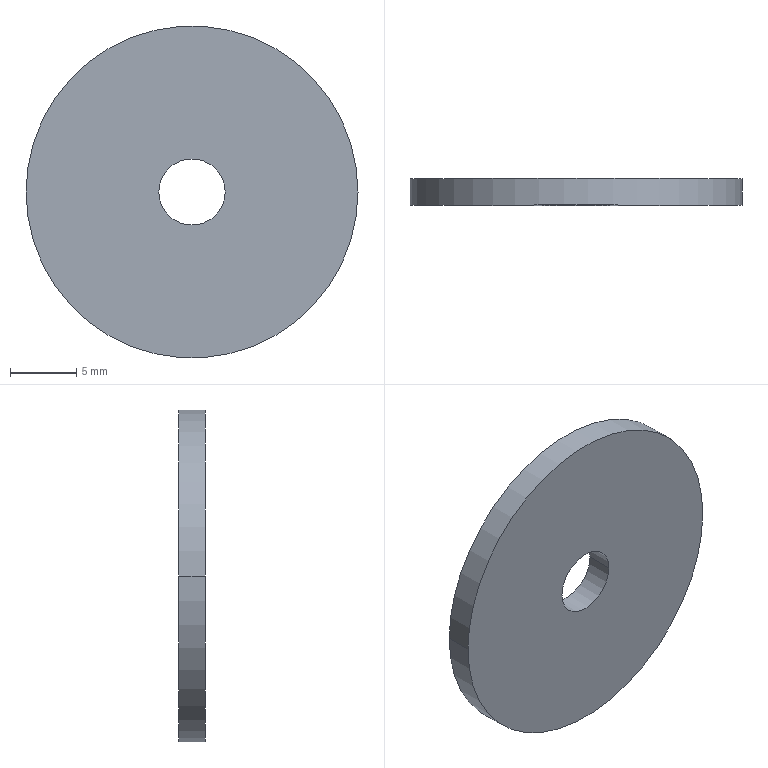Part | STEP file | BAR_INSUL_25 | 1 solid | 6 faces | box 25 x 2 x 25 mm | volume 942.478 mm3 | cylinder 4 | plane 2 | commonest cylinder face diameters 5 x2 25 x2
STEP:
#1=CARTESIAN_POINT('',(0.,0.,0.));
#2=DIRECTION('',(0.,0.,1.));
#3=DIRECTION('',(1.,0.,0.));
#4=AXIS2_PLACEMENT_3D('',#1,#2,#3);
#5=CARTESIAN_POINT('',(-12.5,0.,0.));
#6=VERTEX_POINT('',#5);
#7=CARTESIAN_POINT('',(12.5,0.,0.));
#8=VERTEX_POINT('',#7);
#9=CARTESIAN_POINT('',(0.,0.,0.));
#10=DIRECTION('',(0.,1.,0.));
#11=DIRECTION('',(-1.,0.,0.));
#12=AXIS2_PLACEMENT_3D('',#9,#10,#11);
#13=CIRCLE('',#12,12.5);
#14=CARTESIAN_POINT('',(0.,0.,0.));
#15=DIRECTION('',(0.,1.,0.));
#16=DIRECTION('',(-1.,0.,0.));
#17=AXIS2_PLACEMENT_3D('',#14,#15,#16);
#18=PLANE('',#17);
#19=CARTESIAN_POINT('',(0.,0.));
#20=DIRECTION('',(1.,0.));
#21=AXIS2_PLACEMENT_2D('',#19,#20);
#22=CIRCLE('',#21,12.5);
#23=(GEOMETRIC_REPRESENTATION_CONTEXT(2)PARAMETRIC_REPRESENTATION_CONTEXT()REPRESENTATION_CONTEXT('',''));
#24=DEFINITIONAL_REPRESENTATION('',(#22),#23);
#25=PCURVE('',#18,#24);
#26=CARTESIAN_POINT('',(0.,0.,0.));
#27=DIRECTION('',(0.,1.,0.));
#28=DIRECTION('',(-1.,0.,0.));
#29=AXIS2_PLACEMENT_3D('',#26,#27,#28);
#30=CYLINDRICAL_SURFACE('',#29,12.5);
#31=CARTESIAN_POINT('',(0.,0.));
#32=DIRECTION('',(1.,0.));
#33=VECTOR('',#32,1.);
#34=LINE('',#31,#33);
#35=(GEOMETRIC_REPRESENTATION_CONTEXT(2)PARAMETRIC_REPRESENTATION_CONTEXT()REPRESENTATION_CONTEXT('',''));
#36=DEFINITIONAL_REPRESENTATION('',(#34),#35);
#37=PCURVE('',#30,#36);
#38=SURFACE_CURVE('',#13,(#25,#37),.PCURVE_S1.);
#39=EDGE_CURVE('',#6,#8,#38,.T.);
#40=ORIENTED_EDGE('',*,*,#39,.T.);
#41=CARTESIAN_POINT('',(0.,0.,0.));
#42=DIRECTION('',(0.,1.,0.));
#43=DIRECTION('',(1.,0.,0.));
#44=AXIS2_PLACEMENT_3D('',#41,#42,#43);
#45=CIRCLE('',#44,12.5);
#46=CARTESIAN_POINT('',(0.,0.));
#47=DIRECTION('',(-1.,0.));
#48=AXIS2_PLACEMENT_2D('',#46,#47);
#49=CIRCLE('',#48,12.5);
#50=(GEOMETRIC_REPRESENTATION_CONTEXT(2)PARAMETRIC_REPRESENTATION_CONTEXT()REPRESENTATION_CONTEXT('',''));
#51=DEFINITIONAL_REPRESENTATION('',(#49),#50);
#52=PCURVE('',#18,#51);
#53=CARTESIAN_POINT('',(0.,0.,0.));
#54=DIRECTION('',(0.,1.,0.));
#55=DIRECTION('',(-1.,0.,0.));
#56=AXIS2_PLACEMENT_3D('',#53,#54,#55);
#57=CYLINDRICAL_SURFACE('',#56,12.5);
#58=CARTESIAN_POINT('',(3.142,0.));
#59=DIRECTION('',(1.,0.));
#60=VECTOR('',#59,1.);
#61=LINE('',#58,#60);
#62=(GEOMETRIC_REPRESENTATION_CONTEXT(2)PARAMETRIC_REPRESENTATION_CONTEXT()REPRESENTATION_CONTEXT('',''));
#63=DEFINITIONAL_REPRESENTATION('',(#61),#62);
#64=PCURVE('',#57,#63);
#65=SURFACE_CURVE('',#45,(#52,#64),.PCURVE_S1.);
#66=EDGE_CURVE('',#8,#6,#65,.T.);
#67=ORIENTED_EDGE('',*,*,#66,.T.);
#68=EDGE_LOOP('',(#40,#67));
#69=FACE_BOUND('',#68,.F.);
#70=CARTESIAN_POINT('',(-2.5,0.,0.));
#71=VERTEX_POINT('',#70);
#72=CARTESIAN_POINT('',(2.5,0.,0.));
#73=VERTEX_POINT('',#72);
#74=CARTESIAN_POINT('',(0.,0.,0.));
#75=DIRECTION('',(0.,-1.,0.));
#76=DIRECTION('',(-1.,0.,0.));
#77=AXIS2_PLACEMENT_3D('',#74,#75,#76);
#78=CIRCLE('',#77,2.5);
#79=CARTESIAN_POINT('',(2.5,0.));
#80=CARTESIAN_POINT('',(2.5,-4.33));
#81=CARTESIAN_POINT('',(-1.25,-2.165));
#82=CARTESIAN_POINT('',(-5.,0.));
#83=CARTESIAN_POINT('',(-1.25,2.165));
#84=CARTESIAN_POINT('',(2.5,4.33));
#85=CARTESIAN_POINT('',(2.5,0.));
#86=(BOUNDED_CURVE()B_SPLINE_CURVE(2,(#79,#80,#81,#82,#83,#84,#85),.UNSPECIFIED.,.T.,.F.)B_SPLINE_CURVE_WITH_KNOTS((1,2,2,2,2,1),(-2.094,0.,2.094,4.189,6.283,8.378),.UNSPECIFIED.)CURVE()GEOMETRIC_REPRESENTATION_ITEM()RATIONAL_B_SPLINE_CURVE((1.,0.5,1.,0.5,1.,0.5,1.))REPRESENTATION_ITEM(''));
#87=(GEOMETRIC_REPRESENTATION_CONTEXT(2)PARAMETRIC_REPRESENTATION_CONTEXT()REPRESENTATION_CONTEXT('',''));
#88=DEFINITIONAL_REPRESENTATION('',(#86),#87);
#89=PCURVE('',#18,#88);
#90=CARTESIAN_POINT('',(0.,0.,0.));
#91=DIRECTION('',(0.,1.,0.));
#92=DIRECTION('',(-1.,0.,0.));
#93=AXIS2_PLACEMENT_3D('',#90,#91,#92);
#94=CYLINDRICAL_SURFACE('',#93,2.5);
#95=CARTESIAN_POINT('',(6.283,0.));
#96=DIRECTION('',(-1.,0.));
#97=VECTOR('',#96,1.);
#98=LINE('',#95,#97);
#99=(GEOMETRIC_REPRESENTATION_CONTEXT(2)PARAMETRIC_REPRESENTATION_CONTEXT()REPRESENTATION_CONTEXT('',''));
#100=DEFINITIONAL_REPRESENTATION('',(#98),#99);
#101=PCURVE('',#94,#100);
#102=SURFACE_CURVE('',#78,(#89,#101),.PCURVE_S1.);
#103=EDGE_CURVE('',#71,#73,#102,.T.);
#104=ORIENTED_EDGE('',*,*,#103,.T.);
#105=CARTESIAN_POINT('',(0.,0.,0.));
#106=DIRECTION('',(0.,-1.,0.));
#107=DIRECTION('',(1.,0.,0.));
#108=AXIS2_PLACEMENT_3D('',#105,#106,#107);
#109=CIRCLE('',#108,2.5);
#110=CARTESIAN_POINT('',(-2.5,0.));
#111=CARTESIAN_POINT('',(-2.5,4.33));
#112=CARTESIAN_POINT('',(1.25,2.165));
#113=CARTESIAN_POINT('',(5.,0.));
#114=CARTESIAN_POINT('',(1.25,-2.165));
#115=CARTESIAN_POINT('',(-2.5,-4.33));
#116=CARTESIAN_POINT('',(-2.5,0.));
#117=(BOUNDED_CURVE()B_SPLINE_CURVE(2,(#110,#111,#112,#113,#114,#115,#116),.UNSPECIFIED.,.T.,.F.)B_SPLINE_CURVE_WITH_KNOTS((1,2,2,2,2,1),(-2.094,0.,2.094,4.189,6.283,8.378),.UNSPECIFIED.)CURVE()GEOMETRIC_REPRESENTATION_ITEM()RATIONAL_B_SPLINE_CURVE((1.,0.5,1.,0.5,1.,0.5,1.))REPRESENTATION_ITEM(''));
#118=(GEOMETRIC_REPRESENTATION_CONTEXT(2)PARAMETRIC_REPRESENTATION_CONTEXT()REPRESENTATION_CONTEXT('',''));
#119=DEFINITIONAL_REPRESENTATION('',(#117),#118);
#120=PCURVE('',#18,#119);
#121=CARTESIAN_POINT('',(0.,0.,0.));
#122=DIRECTION('',(0.,1.,0.));
#123=DIRECTION('',(-1.,0.,0.));
#124=AXIS2_PLACEMENT_3D('',#121,#122,#123);
#125=CYLINDRICAL_SURFACE('',#124,2.5);
#126=CARTESIAN_POINT('',(3.142,0.));
#127=DIRECTION('',(-1.,0.));
#128=VECTOR('',#127,1.);
#129=LINE('',#126,#128);
#130=(GEOMETRIC_REPRESENTATION_CONTEXT(2)PARAMETRIC_REPRESENTATION_CONTEXT()REPRESENTATION_CONTEXT('',''));
#131=DEFINITIONAL_REPRESENTATION('',(#129),#130);
#132=PCURVE('',#125,#131);
#133=SURFACE_CURVE('',#109,(#120,#132),.PCURVE_S1.);
#134=EDGE_CURVE('',#73,#71,#133,.T.);
#135=ORIENTED_EDGE('',*,*,#134,.T.);
#136=EDGE_LOOP('',(#104,#135));
#137=FACE_BOUND('',#136,.F.);
#138=ADVANCED_FACE('',(#69,#137),#18,.F.);
#139=CARTESIAN_POINT('',(12.5,2.,0.));
#140=VERTEX_POINT('',#139);
#141=CARTESIAN_POINT('',(12.5,0.,0.));
#142=DIRECTION('',(0.,1.,0.));
#143=VECTOR('',#142,1.);
#144=LINE('',#141,#143);
#145=CARTESIAN_POINT('',(3.142,0.));
#146=DIRECTION('',(0.,1.));
#147=VECTOR('',#146,1.);
#148=LINE('',#145,#147);
#149=(GEOMETRIC_REPRESENTATION_CONTEXT(2)PARAMETRIC_REPRESENTATION_CONTEXT()REPRESENTATION_CONTEXT('',''));
#150=DEFINITIONAL_REPRESENTATION('',(#148),#149);
#151=PCURVE('',#30,#150);
#152=CARTESIAN_POINT('',(3.142,0.));
#153=DIRECTION('',(0.,1.));
#154=VECTOR('',#153,1.);
#155=LINE('',#152,#154);
#156=(GEOMETRIC_REPRESENTATION_CONTEXT(2)PARAMETRIC_REPRESENTATION_CONTEXT()REPRESENTATION_CONTEXT('',''));
#157=DEFINITIONAL_REPRESENTATION('',(#155),#156);
#158=PCURVE('',#57,#157);
#159=SURFACE_CURVE('',#144,(#151,#158),.PCURVE_S1.);
#160=EDGE_CURVE('',#8,#140,#159,.T.);
#161=ORIENTED_EDGE('',*,*,#160,.T.);
#162=CARTESIAN_POINT('',(-12.5,2.,0.));
#163=VERTEX_POINT('',#162);
#164=CARTESIAN_POINT('',(0.,2.,0.));
#165=DIRECTION('',(0.,1.,0.));
#166=DIRECTION('',(-1.,0.,0.));
#167=AXIS2_PLACEMENT_3D('',#164,#165,#166);
#168=CIRCLE('',#167,12.5);
#169=CARTESIAN_POINT('',(0.,2.));
#170=DIRECTION('',(1.,0.));
#171=VECTOR('',#170,1.);
#172=LINE('',#169,#171);
#173=(GEOMETRIC_REPRESENTATION_CONTEXT(2)PARAMETRIC_REPRESENTATION_CONTEXT()REPRESENTATION_CONTEXT('',''));
#174=DEFINITIONAL_REPRESENTATION('',(#172),#173);
#175=PCURVE('',#30,#174);
#176=CARTESIAN_POINT('',(0.,2.,0.));
#177=DIRECTION('',(0.,1.,0.));
#178=DIRECTION('',(-1.,0.,0.));
#179=AXIS2_PLACEMENT_3D('',#176,#177,#178);
#180=PLANE('',#179);
#181=CARTESIAN_POINT('',(0.,0.));
#182=DIRECTION('',(1.,0.));
#183=AXIS2_PLACEMENT_2D('',#181,#182);
#184=CIRCLE('',#183,12.5);
#185=(GEOMETRIC_REPRESENTATION_CONTEXT(2)PARAMETRIC_REPRESENTATION_CONTEXT()REPRESENTATION_CONTEXT('',''));
#186=DEFINITIONAL_REPRESENTATION('',(#184),#185);
#187=PCURVE('',#180,#186);
#188=SURFACE_CURVE('',#168,(#175,#187),.PCURVE_S1.);
#189=EDGE_CURVE('',#163,#140,#188,.T.);
#190=ORIENTED_EDGE('',*,*,#189,.F.);
#191=CARTESIAN_POINT('',(-12.5,0.,0.));
#192=DIRECTION('',(0.,1.,0.));
#193=VECTOR('',#192,1.);
#194=LINE('',#191,#193);
#195=CARTESIAN_POINT('',(0.,0.));
#196=DIRECTION('',(0.,1.));
#197=VECTOR('',#196,1.);
#198=LINE('',#195,#197);
#199=(GEOMETRIC_REPRESENTATION_CONTEXT(2)PARAMETRIC_REPRESENTATION_CONTEXT()REPRESENTATION_CONTEXT('',''));
#200=DEFINITIONAL_REPRESENTATION('',(#198),#199);
#201=PCURVE('',#30,#200);
#202=CARTESIAN_POINT('',(6.283,0.));
#203=DIRECTION('',(0.,1.));
#204=VECTOR('',#203,1.);
#205=LINE('',#202,#204);
#206=(GEOMETRIC_REPRESENTATION_CONTEXT(2)PARAMETRIC_REPRESENTATION_CONTEXT()REPRESENTATION_CONTEXT('',''));
#207=DEFINITIONAL_REPRESENTATION('',(#205),#206);
#208=PCURVE('',#57,#207);
#209=SURFACE_CURVE('',#194,(#201,#208),.PCURVE_S1.);
#210=EDGE_CURVE('',#6,#163,#209,.T.);
#211=ORIENTED_EDGE('',*,*,#210,.F.);
#212=ORIENTED_EDGE('',*,*,#39,.T.);
#213=EDGE_LOOP('',(#161,#190,#211,#212));
#214=FACE_BOUND('',#213,.T.);
#215=ADVANCED_FACE('',(#214),#30,.T.);
#216=ORIENTED_EDGE('',*,*,#210,.T.);
#217=CARTESIAN_POINT('',(0.,2.,0.));
#218=DIRECTION('',(0.,1.,0.));
#219=DIRECTION('',(1.,0.,0.));
#220=AXIS2_PLACEMENT_3D('',#217,#218,#219);
#221=CIRCLE('',#220,12.5);
#222=CARTESIAN_POINT('',(3.142,2.));
#223=DIRECTION('',(1.,0.));
#224=VECTOR('',#223,1.);
#225=LINE('',#222,#224);
#226=(GEOMETRIC_REPRESENTATION_CONTEXT(2)PARAMETRIC_REPRESENTATION_CONTEXT()REPRESENTATION_CONTEXT('',''));
#227=DEFINITIONAL_REPRESENTATION('',(#225),#226);
#228=PCURVE('',#57,#227);
#229=CARTESIAN_POINT('',(0.,0.));
#230=DIRECTION('',(-1.,0.));
#231=AXIS2_PLACEMENT_2D('',#229,#230);
#232=CIRCLE('',#231,12.5);
#233=(GEOMETRIC_REPRESENTATION_CONTEXT(2)PARAMETRIC_REPRESENTATION_CONTEXT()REPRESENTATION_CONTEXT('',''));
#234=DEFINITIONAL_REPRESENTATION('',(#232),#233);
#235=PCURVE('',#180,#234);
#236=SURFACE_CURVE('',#221,(#228,#235),.PCURVE_S1.);
#237=EDGE_CURVE('',#140,#163,#236,.T.);
#238=ORIENTED_EDGE('',*,*,#237,.F.);
#239=ORIENTED_EDGE('',*,*,#160,.F.);
#240=ORIENTED_EDGE('',*,*,#66,.T.);
#241=EDGE_LOOP('',(#216,#238,#239,#240));
#242=FACE_BOUND('',#241,.T.);
#243=ADVANCED_FACE('',(#242),#57,.T.);
#244=ORIENTED_EDGE('',*,*,#189,.F.);
#245=ORIENTED_EDGE('',*,*,#237,.F.);
#246=EDGE_LOOP('',(#244,#245));
#247=FACE_BOUND('',#246,.F.);
#248=CARTESIAN_POINT('',(-2.5,2.,0.));
#249=VERTEX_POINT('',#248);
#250=CARTESIAN_POINT('',(2.5,2.,0.));
#251=VERTEX_POINT('',#250);
#252=CARTESIAN_POINT('',(0.,2.,0.));
#253=DIRECTION('',(0.,-1.,0.));
#254=DIRECTION('',(-1.,0.,0.));
#255=AXIS2_PLACEMENT_3D('',#252,#253,#254);
#256=CIRCLE('',#255,2.5);
#257=CARTESIAN_POINT('',(2.5,0.));
#258=CARTESIAN_POINT('',(2.5,-4.33));
#259=CARTESIAN_POINT('',(-1.25,-2.165));
#260=CARTESIAN_POINT('',(-5.,0.));
#261=CARTESIAN_POINT('',(-1.25,2.165));
#262=CARTESIAN_POINT('',(2.5,4.33));
#263=CARTESIAN_POINT('',(2.5,0.));
#264=(BOUNDED_CURVE()B_SPLINE_CURVE(2,(#257,#258,#259,#260,#261,#262,#263),.UNSPECIFIED.,.T.,.F.)B_SPLINE_CURVE_WITH_KNOTS((1,2,2,2,2,1),(-2.094,0.,2.094,4.189,6.283,8.378),.UNSPECIFIED.)CURVE()GEOMETRIC_REPRESENTATION_ITEM()RATIONAL_B_SPLINE_CURVE((1.,0.5,1.,0.5,1.,0.5,1.))REPRESENTATION_ITEM(''));
#265=(GEOMETRIC_REPRESENTATION_CONTEXT(2)PARAMETRIC_REPRESENTATION_CONTEXT()REPRESENTATION_CONTEXT('',''));
#266=DEFINITIONAL_REPRESENTATION('',(#264),#265);
#267=PCURVE('',#180,#266);
#268=CARTESIAN_POINT('',(6.283,2.));
#269=DIRECTION('',(-1.,0.));
#270=VECTOR('',#269,1.);
#271=LINE('',#268,#270);
#272=(GEOMETRIC_REPRESENTATION_CONTEXT(2)PARAMETRIC_REPRESENTATION_CONTEXT()REPRESENTATION_CONTEXT('',''));
#273=DEFINITIONAL_REPRESENTATION('',(#271),#272);
#274=PCURVE('',#94,#273);
#275=SURFACE_CURVE('',#256,(#267,#274),.PCURVE_S1.);
#276=EDGE_CURVE('',#249,#251,#275,.T.);
#277=ORIENTED_EDGE('',*,*,#276,.F.);
#278=CARTESIAN_POINT('',(0.,2.,0.));
#279=DIRECTION('',(0.,-1.,0.));
#280=DIRECTION('',(1.,0.,0.));
#281=AXIS2_PLACEMENT_3D('',#278,#279,#280);
#282=CIRCLE('',#281,2.5);
#283=CARTESIAN_POINT('',(-2.5,0.));
#284=CARTESIAN_POINT('',(-2.5,4.33));
#285=CARTESIAN_POINT('',(1.25,2.165));
#286=CARTESIAN_POINT('',(5.,0.));
#287=CARTESIAN_POINT('',(1.25,-2.165));
#288=CARTESIAN_POINT('',(-2.5,-4.33));
#289=CARTESIAN_POINT('',(-2.5,0.));
#290=(BOUNDED_CURVE()B_SPLINE_CURVE(2,(#283,#284,#285,#286,#287,#288,#289),.UNSPECIFIED.,.T.,.F.)B_SPLINE_CURVE_WITH_KNOTS((1,2,2,2,2,1),(-2.094,0.,2.094,4.189,6.283,8.378),.UNSPECIFIED.)CURVE()GEOMETRIC_REPRESENTATION_ITEM()RATIONAL_B_SPLINE_CURVE((1.,0.5,1.,0.5,1.,0.5,1.))REPRESENTATION_ITEM(''));
#291=(GEOMETRIC_REPRESENTATION_CONTEXT(2)PARAMETRIC_REPRESENTATION_CONTEXT()REPRESENTATION_CONTEXT('',''));
#292=DEFINITIONAL_REPRESENTATION('',(#290),#291);
#293=PCURVE('',#180,#292);
#294=CARTESIAN_POINT('',(3.142,2.));
#295=DIRECTION('',(-1.,0.));
#296=VECTOR('',#295,1.);
#297=LINE('',#294,#296);
#298=(GEOMETRIC_REPRESENTATION_CONTEXT(2)PARAMETRIC_REPRESENTATION_CONTEXT()REPRESENTATION_CONTEXT('',''));
#299=DEFINITIONAL_REPRESENTATION('',(#297),#298);
#300=PCURVE('',#125,#299);
#301=SURFACE_CURVE('',#282,(#293,#300),.PCURVE_S1.);
#302=EDGE_CURVE('',#251,#249,#301,.T.);
#303=ORIENTED_EDGE('',*,*,#302,.F.);
#304=EDGE_LOOP('',(#277,#303));
#305=FACE_BOUND('',#304,.F.);
#306=ADVANCED_FACE('',(#247,#305),#180,.T.);
#307=ORIENTED_EDGE('',*,*,#103,.F.);
#308=CARTESIAN_POINT('',(-2.5,0.,0.));
#309=DIRECTION('',(0.,1.,0.));
#310=VECTOR('',#309,1.);
#311=LINE('',#308,#310);
#312=CARTESIAN_POINT('',(6.283,0.));
#313=DIRECTION('',(0.,1.));
#314=VECTOR('',#313,1.);
#315=LINE('',#312,#314);
#316=(GEOMETRIC_REPRESENTATION_CONTEXT(2)PARAMETRIC_REPRESENTATION_CONTEXT()REPRESENTATION_CONTEXT('',''));
#317=DEFINITIONAL_REPRESENTATION('',(#315),#316);
#318=PCURVE('',#94,#317);
#319=CARTESIAN_POINT('',(0.,0.));
#320=DIRECTION('',(0.,1.));
#321=VECTOR('',#320,1.);
#322=LINE('',#319,#321);
#323=(GEOMETRIC_REPRESENTATION_CONTEXT(2)PARAMETRIC_REPRESENTATION_CONTEXT()REPRESENTATION_CONTEXT('',''));
#324=DEFINITIONAL_REPRESENTATION('',(#322),#323);
#325=PCURVE('',#125,#324);
#326=SURFACE_CURVE('',#311,(#318,#325),.PCURVE_S1.);
#327=EDGE_CURVE('',#71,#249,#326,.T.);
#328=ORIENTED_EDGE('',*,*,#327,.T.);
#329=ORIENTED_EDGE('',*,*,#276,.T.);
#330=CARTESIAN_POINT('',(2.5,0.,0.));
#331=DIRECTION('',(0.,1.,0.));
#332=VECTOR('',#331,1.);
#333=LINE('',#330,#332);
#334=CARTESIAN_POINT('',(3.142,0.));
#335=DIRECTION('',(0.,1.));
#336=VECTOR('',#335,1.);
#337=LINE('',#334,#336);
#338=(GEOMETRIC_REPRESENTATION_CONTEXT(2)PARAMETRIC_REPRESENTATION_CONTEXT()REPRESENTATION_CONTEXT('',''));
#339=DEFINITIONAL_REPRESENTATION('',(#337),#338);
#340=PCURVE('',#94,#339);
#341=CARTESIAN_POINT('',(3.142,0.));
#342=DIRECTION('',(0.,1.));
#343=VECTOR('',#342,1.);
#344=LINE('',#341,#343);
#345=(GEOMETRIC_REPRESENTATION_CONTEXT(2)PARAMETRIC_REPRESENTATION_CONTEXT()REPRESENTATION_CONTEXT('',''));
#346=DEFINITIONAL_REPRESENTATION('',(#344),#345);
#347=PCURVE('',#125,#346);
#348=SURFACE_CURVE('',#333,(#340,#347),.PCURVE_S1.);
#349=EDGE_CURVE('',#73,#251,#348,.T.);
#350=ORIENTED_EDGE('',*,*,#349,.F.);
#351=EDGE_LOOP('',(#307,#328,#329,#350));
#352=FACE_BOUND('',#351,.F.);
#353=ADVANCED_FACE('',(#352),#94,.F.);
#354=ORIENTED_EDGE('',*,*,#134,.F.);
#355=ORIENTED_EDGE('',*,*,#349,.T.);
#356=ORIENTED_EDGE('',*,*,#302,.T.);
#357=ORIENTED_EDGE('',*,*,#327,.F.);
#358=EDGE_LOOP('',(#354,#355,#356,#357));
#359=FACE_BOUND('',#358,.F.);
#360=ADVANCED_FACE('',(#359),#125,.F.);
#361=CLOSED_SHELL('',(#138,#215,#243,#306,#353,#360));
#362=MANIFOLD_SOLID_BREP('',#361);
#363=(LENGTH_UNIT()NAMED_UNIT(*)SI_UNIT(.MILLI.,.METRE.));
#364=UNCERTAINTY_MEASURE_WITH_UNIT(LENGTH_MEASURE(0.0000001),#363,'','');
#365=(NAMED_UNIT(*)PLANE_ANGLE_UNIT()SI_UNIT($,.RADIAN.));
#366=(NAMED_UNIT(*)SI_UNIT($,.STERADIAN.)SOLID_ANGLE_UNIT());
#367=(GEOMETRIC_REPRESENTATION_CONTEXT(3)GLOBAL_UNCERTAINTY_ASSIGNED_CONTEXT((#364))GLOBAL_UNIT_ASSIGNED_CONTEXT((#363,#365,#366))REPRESENTATION_CONTEXT('',''));
#368=ADVANCED_BREP_SHAPE_REPRESENTATION('',(#4,#362),#367);